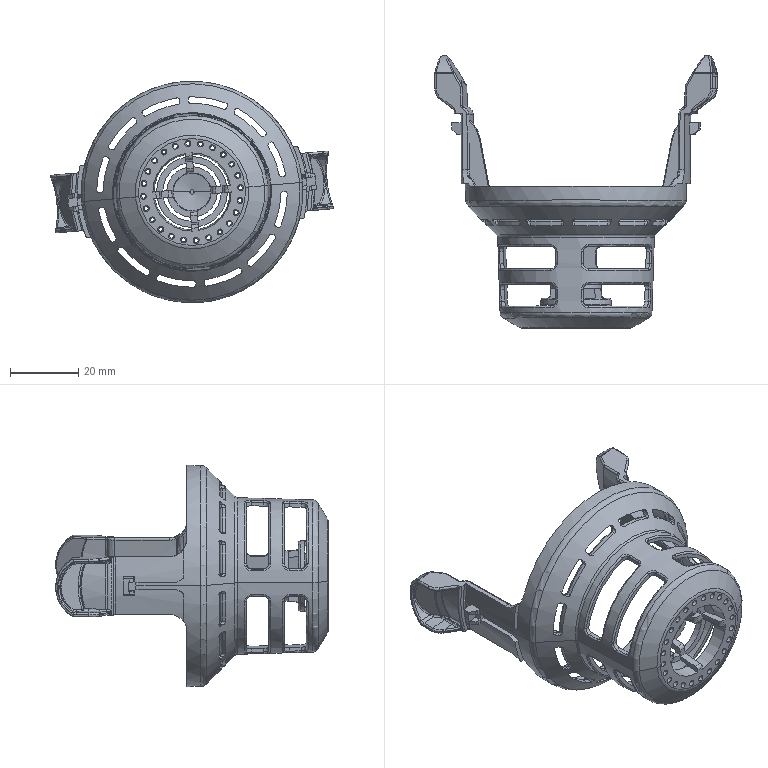Part | STEP file | ZXW722-L-11 | 1 solid | 749 faces | box 82.99 x 80.1 x 65 mm | volume 13672 mm3 | spline 250 | cylinder 144 | plane 121 | cone 112 | torus 90 | other 20 | sphere 12 | commonest cylinder face diameters 1.4 x48 1 x36 1.2 x24 3 x8 71.6 x6 0.4 x4